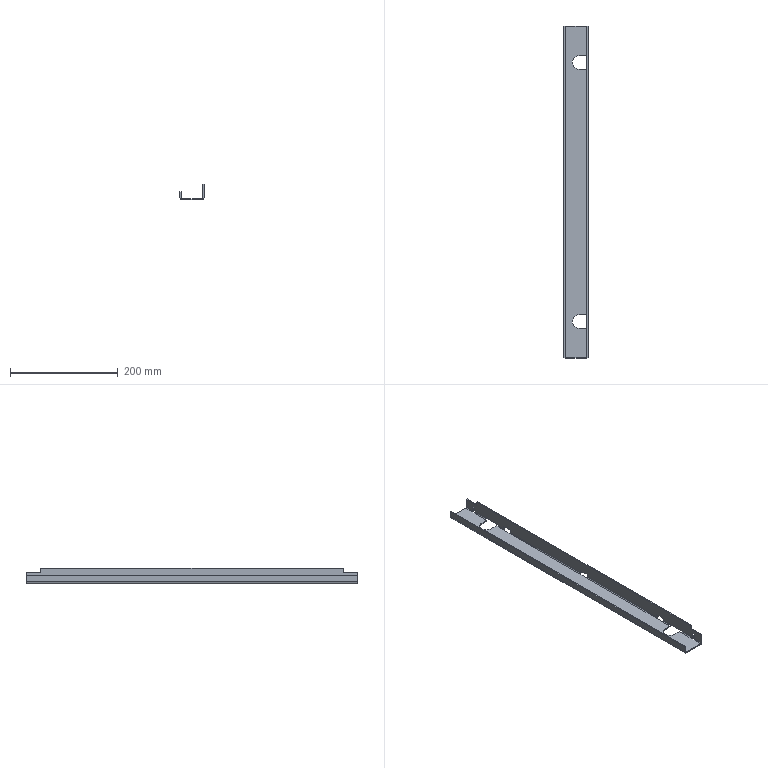Part | STEP file | Instrument door gasket strip vertical (lock hole) modified | 1 solid | 89 faces | box 44.5 x 615 x 28.5 mm | volume 95558 mm3 | plane 67 | cylinder 22 | commonest cylinder face diameters 3 x9 7 x9 25 x4